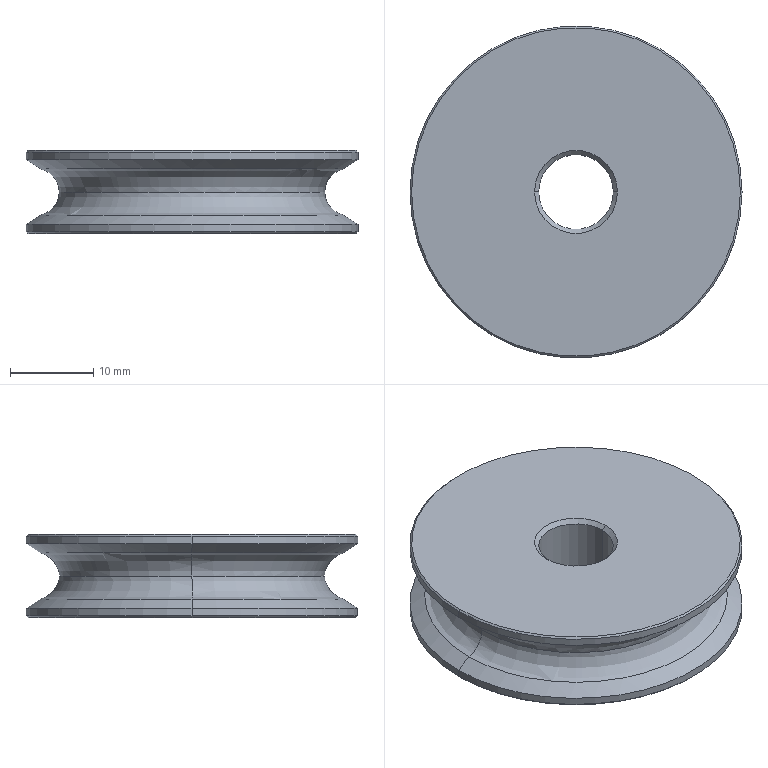Part | STEP file | 10000020591swp000-1 | 1 solid | 24 faces | box 40 x 40 x 10 mm | volume 9487 mm3 | cone 12 | cylinder 6 | torus 4 | plane 2 | commonest cylinder face diameters 40 x4 9 x2
STEP:
#1=CARTESIAN_POINT('',(-4.5,0.,4.5));
#2=VERTEX_POINT('',#1);
#3=CARTESIAN_POINT('',(4.5,0.,4.5));
#4=VERTEX_POINT('',#3);
#5=CARTESIAN_POINT('',(0.,0.,4.5));
#6=DIRECTION('',(0.,0.,1.));
#7=DIRECTION('',(1.,0.,0.));
#8=AXIS2_PLACEMENT_3D('',#5,#6,#7);
#9=CIRCLE('',#8,4.5);
#10=EDGE_CURVE('',#2,#4,#9,.T.);
#11=ORIENTED_EDGE('',*,*,#10,.F.);
#12=CARTESIAN_POINT('',(-5.,0.,5.));
#13=VERTEX_POINT('',#12);
#14=CARTESIAN_POINT('',(-4.5,0.,4.5));
#15=DIRECTION('',(-0.7071,0.,0.7071));
#16=VECTOR('',#15,1000.);
#17=LINE('',#14,#16);
#18=EDGE_CURVE('',#2,#13,#17,.T.);
#19=ORIENTED_EDGE('',*,*,#18,.T.);
#20=CARTESIAN_POINT('',(5.,0.,5.));
#21=VERTEX_POINT('',#20);
#22=CARTESIAN_POINT('',(0.,0.,5.));
#23=DIRECTION('',(0.,0.,-1.));
#24=DIRECTION('',(1.,0.,0.));
#25=AXIS2_PLACEMENT_3D('',#22,#23,#24);
#26=CIRCLE('',#25,5.);
#27=EDGE_CURVE('',#21,#13,#26,.T.);
#28=ORIENTED_EDGE('',*,*,#27,.F.);
#29=CARTESIAN_POINT('',(4.5,0.,4.5));
#30=DIRECTION('',(0.7071,0.,0.7071));
#31=VECTOR('',#30,1000.);
#32=LINE('',#29,#31);
#33=EDGE_CURVE('',#4,#21,#32,.T.);
#34=ORIENTED_EDGE('',*,*,#33,.F.);
#35=EDGE_LOOP('',(#11,#19,#28,#34));
#36=FACE_OUTER_BOUND('',#35,.T.);
#37=CARTESIAN_POINT('',(0.,0.,4.5));
#38=DIRECTION('',(0.,0.,1.));
#39=DIRECTION('',(1.,0.,0.));
#40=AXIS2_PLACEMENT_3D('',#37,#38,#39);
#41=CONICAL_SURFACE('',#40,4.5,0.7854);
#42=ADVANCED_FACE('',(#36),#41,.F.);
#43=CARTESIAN_POINT('',(4.5,0.,-4.5));
#44=VERTEX_POINT('',#43);
#45=CARTESIAN_POINT('',(-4.5,0.,-4.5));
#46=VERTEX_POINT('',#45);
#47=CARTESIAN_POINT('',(0.,0.,-4.5));
#48=DIRECTION('',(0.,0.,-1.));
#49=DIRECTION('',(1.,0.,0.));
#50=AXIS2_PLACEMENT_3D('',#47,#48,#49);
#51=CIRCLE('',#50,4.5);
#52=EDGE_CURVE('',#44,#46,#51,.T.);
#53=ORIENTED_EDGE('',*,*,#52,.F.);
#54=CARTESIAN_POINT('',(5.,0.,-5.));
#55=VERTEX_POINT('',#54);
#56=CARTESIAN_POINT('',(5.,0.,-5.));
#57=DIRECTION('',(0.7071,0.,-0.7071));
#58=VECTOR('',#57,1000.);
#59=LINE('',#56,#58);
#60=EDGE_CURVE('',#44,#55,#59,.T.);
#61=ORIENTED_EDGE('',*,*,#60,.T.);
#62=CARTESIAN_POINT('',(-5.,0.,-5.));
#63=VERTEX_POINT('',#62);
#64=CARTESIAN_POINT('',(0.,0.,-5.));
#65=DIRECTION('',(0.,0.,1.));
#66=DIRECTION('',(1.,0.,0.));
#67=AXIS2_PLACEMENT_3D('',#64,#65,#66);
#68=CIRCLE('',#67,5.);
#69=EDGE_CURVE('',#63,#55,#68,.T.);
#70=ORIENTED_EDGE('',*,*,#69,.F.);
#71=CARTESIAN_POINT('',(-5.,0.,-5.));
#72=DIRECTION('',(-0.7071,0.,-0.7071));
#73=VECTOR('',#72,1000.);
#74=LINE('',#71,#73);
#75=EDGE_CURVE('',#46,#63,#74,.T.);
#76=ORIENTED_EDGE('',*,*,#75,.F.);
#77=EDGE_LOOP('',(#53,#61,#70,#76));
#78=FACE_OUTER_BOUND('',#77,.T.);
#79=CARTESIAN_POINT('',(0.,0.,-5.));
#80=DIRECTION('',(0.,0.,-1.));
#81=DIRECTION('',(-1.,0.,0.));
#82=AXIS2_PLACEMENT_3D('',#79,#80,#81);
#83=CONICAL_SURFACE('',#82,5.,0.7854);
#84=ADVANCED_FACE('',(#78),#83,.F.);
#85=CARTESIAN_POINT('',(-19.8,0.,-5.));
#86=VERTEX_POINT('',#85);
#87=CARTESIAN_POINT('',(19.8,0.,-5.));
#88=VERTEX_POINT('',#87);
#89=CARTESIAN_POINT('',(0.,0.,-5.));
#90=DIRECTION('',(0.,0.,-1.));
#91=DIRECTION('',(1.,0.,0.));
#92=AXIS2_PLACEMENT_3D('',#89,#90,#91);
#93=CIRCLE('',#92,19.8);
#94=EDGE_CURVE('',#86,#88,#93,.T.);
#95=ORIENTED_EDGE('',*,*,#94,.F.);
#96=CARTESIAN_POINT('',(-20.,0.,-4.8));
#97=VERTEX_POINT('',#96);
#98=CARTESIAN_POINT('',(-20.,0.,-4.8));
#99=DIRECTION('',(-0.7071,0.,0.7071));
#100=VECTOR('',#99,1000.);
#101=LINE('',#98,#100);
#102=EDGE_CURVE('',#86,#97,#101,.T.);
#103=ORIENTED_EDGE('',*,*,#102,.T.);
#104=CARTESIAN_POINT('',(20.,0.,-4.8));
#105=VERTEX_POINT('',#104);
#106=CARTESIAN_POINT('',(0.,0.,-4.8));
#107=DIRECTION('',(0.,0.,1.));
#108=DIRECTION('',(1.,0.,0.));
#109=AXIS2_PLACEMENT_3D('',#106,#107,#108);
#110=CIRCLE('',#109,20.);
#111=EDGE_CURVE('',#105,#97,#110,.T.);
#112=ORIENTED_EDGE('',*,*,#111,.F.);
#113=CARTESIAN_POINT('',(20.,0.,-4.8));
#114=DIRECTION('',(0.7071,0.,0.7071));
#115=VECTOR('',#114,1000.);
#116=LINE('',#113,#115);
#117=EDGE_CURVE('',#88,#105,#116,.T.);
#118=ORIENTED_EDGE('',*,*,#117,.F.);
#119=EDGE_LOOP('',(#95,#103,#112,#118));
#120=FACE_OUTER_BOUND('',#119,.T.);
#121=CARTESIAN_POINT('',(0.,0.,-4.8));
#122=DIRECTION('',(0.,0.,1.));
#123=DIRECTION('',(1.,0.,0.));
#124=AXIS2_PLACEMENT_3D('',#121,#122,#123);
#125=CONICAL_SURFACE('',#124,20.,0.7854);
#126=ADVANCED_FACE('',(#120),#125,.T.);
#127=CARTESIAN_POINT('',(19.8,0.,5.));
#128=VERTEX_POINT('',#127);
#129=CARTESIAN_POINT('',(-19.8,0.,5.));
#130=VERTEX_POINT('',#129);
#131=CARTESIAN_POINT('',(0.,0.,5.));
#132=DIRECTION('',(0.,0.,1.));
#133=DIRECTION('',(1.,0.,0.));
#134=AXIS2_PLACEMENT_3D('',#131,#132,#133);
#135=CIRCLE('',#134,19.8);
#136=EDGE_CURVE('',#128,#130,#135,.T.);
#137=ORIENTED_EDGE('',*,*,#136,.F.);
#138=CARTESIAN_POINT('',(20.,0.,4.8));
#139=VERTEX_POINT('',#138);
#140=CARTESIAN_POINT('',(19.8,0.,5.));
#141=DIRECTION('',(0.7071,0.,-0.7071));
#142=VECTOR('',#141,1000.);
#143=LINE('',#140,#142);
#144=EDGE_CURVE('',#128,#139,#143,.T.);
#145=ORIENTED_EDGE('',*,*,#144,.T.);
#146=CARTESIAN_POINT('',(-20.,0.,4.8));
#147=VERTEX_POINT('',#146);
#148=CARTESIAN_POINT('',(0.,0.,4.8));
#149=DIRECTION('',(0.,0.,-1.));
#150=DIRECTION('',(1.,0.,0.));
#151=AXIS2_PLACEMENT_3D('',#148,#149,#150);
#152=CIRCLE('',#151,20.);
#153=EDGE_CURVE('',#147,#139,#152,.T.);
#154=ORIENTED_EDGE('',*,*,#153,.F.);
#155=CARTESIAN_POINT('',(-19.8,0.,5.));
#156=DIRECTION('',(-0.7071,0.,-0.7071));
#157=VECTOR('',#156,1000.);
#158=LINE('',#155,#157);
#159=EDGE_CURVE('',#130,#147,#158,.T.);
#160=ORIENTED_EDGE('',*,*,#159,.F.);
#161=EDGE_LOOP('',(#137,#145,#154,#160));
#162=FACE_OUTER_BOUND('',#161,.T.);
#163=CARTESIAN_POINT('',(0.,0.,5.));
#164=DIRECTION('',(0.,0.,-1.));
#165=DIRECTION('',(-1.,0.,0.));
#166=AXIS2_PLACEMENT_3D('',#163,#164,#165);
#167=CONICAL_SURFACE('',#166,19.8,0.7854);
#168=ADVANCED_FACE('',(#162),#167,.T.);
#169=CARTESIAN_POINT('',(-18.244,0.,2.785));
#170=VERTEX_POINT('',#169);
#171=CARTESIAN_POINT('',(18.244,0.,2.785));
#172=VERTEX_POINT('',#171);
#173=CARTESIAN_POINT('',(0.,0.,2.785));
#174=DIRECTION('',(0.,0.,-1.));
#175=DIRECTION('',(-1.,0.,0.));
#176=AXIS2_PLACEMENT_3D('',#173,#174,#175);
#177=CIRCLE('',#176,18.244);
#178=EDGE_CURVE('',#170,#172,#177,.T.);
#179=ORIENTED_EDGE('',*,*,#178,.F.);
#180=CARTESIAN_POINT('',(-20.,0.,3.909));
#181=VERTEX_POINT('',#180);
#182=CARTESIAN_POINT('',(-20.,0.,3.909));
#183=DIRECTION('',(-0.8422,0.,0.5391));
#184=VECTOR('',#183,1000.);
#185=LINE('',#182,#184);
#186=EDGE_CURVE('',#170,#181,#185,.T.);
#187=ORIENTED_EDGE('',*,*,#186,.T.);
#188=CARTESIAN_POINT('',(20.,0.,3.909));
#189=VERTEX_POINT('',#188);
#190=CARTESIAN_POINT('',(0.,0.,3.909));
#191=DIRECTION('',(0.,0.,1.));
#192=DIRECTION('',(1.,0.,0.));
#193=AXIS2_PLACEMENT_3D('',#190,#191,#192);
#194=CIRCLE('',#193,20.);
#195=EDGE_CURVE('',#189,#181,#194,.T.);
#196=ORIENTED_EDGE('',*,*,#195,.F.);
#197=CARTESIAN_POINT('',(20.,0.,3.909));
#198=DIRECTION('',(0.8422,0.,0.5391));
#199=VECTOR('',#198,1000.);
#200=LINE('',#197,#199);
#201=EDGE_CURVE('',#172,#189,#200,.T.);
#202=ORIENTED_EDGE('',*,*,#201,.F.);
#203=EDGE_LOOP('',(#179,#187,#196,#202));
#204=FACE_OUTER_BOUND('',#203,.T.);
#205=CARTESIAN_POINT('',(0.,0.,3.909));
#206=DIRECTION('',(0.,0.,1.));
#207=DIRECTION('',(1.,0.,0.));
#208=AXIS2_PLACEMENT_3D('',#205,#206,#207);
#209=CONICAL_SURFACE('',#208,20.,1.001);
#210=ADVANCED_FACE('',(#204),#209,.T.);
#211=CARTESIAN_POINT('',(18.244,0.,-2.785));
#212=VERTEX_POINT('',#211);
#213=CARTESIAN_POINT('',(-18.244,0.,-2.785));
#214=VERTEX_POINT('',#213);
#215=CARTESIAN_POINT('',(0.,0.,-2.785));
#216=DIRECTION('',(0.,0.,1.));
#217=DIRECTION('',(1.,0.,0.));
#218=AXIS2_PLACEMENT_3D('',#215,#216,#217);
#219=CIRCLE('',#218,18.244);
#220=EDGE_CURVE('',#212,#214,#219,.T.);
#221=ORIENTED_EDGE('',*,*,#220,.F.);
#222=CARTESIAN_POINT('',(20.,0.,-3.909));
#223=VERTEX_POINT('',#222);
#224=CARTESIAN_POINT('',(18.244,0.,-2.785));
#225=DIRECTION('',(0.8422,0.,-0.5391));
#226=VECTOR('',#225,1000.);
#227=LINE('',#224,#226);
#228=EDGE_CURVE('',#212,#223,#227,.T.);
#229=ORIENTED_EDGE('',*,*,#228,.T.);
#230=CARTESIAN_POINT('',(-20.,0.,-3.909));
#231=VERTEX_POINT('',#230);
#232=CARTESIAN_POINT('',(0.,0.,-3.909));
#233=DIRECTION('',(0.,0.,-1.));
#234=DIRECTION('',(-1.,0.,0.));
#235=AXIS2_PLACEMENT_3D('',#232,#233,#234);
#236=CIRCLE('',#235,20.);
#237=EDGE_CURVE('',#231,#223,#236,.T.);
#238=ORIENTED_EDGE('',*,*,#237,.F.);
#239=CARTESIAN_POINT('',(-18.244,0.,-2.785));
#240=DIRECTION('',(-0.8422,0.,-0.5391));
#241=VECTOR('',#240,1000.);
#242=LINE('',#239,#241);
#243=EDGE_CURVE('',#214,#231,#242,.T.);
#244=ORIENTED_EDGE('',*,*,#243,.F.);
#245=EDGE_LOOP('',(#221,#229,#238,#244));
#246=FACE_OUTER_BOUND('',#245,.T.);
#247=CARTESIAN_POINT('',(0.,0.,-2.785));
#248=DIRECTION('',(0.,0.,-1.));
#249=DIRECTION('',(-1.,0.,0.));
#250=AXIS2_PLACEMENT_3D('',#247,#248,#249);
#251=CONICAL_SURFACE('',#250,18.244,1.001);
#252=ADVANCED_FACE('',(#246),#251,.T.);
#253=CARTESIAN_POINT('',(0.,0.,-2.785));
#254=DIRECTION('',(0.,0.,1.));
#255=DIRECTION('',(1.,0.,0.));
#256=AXIS2_PLACEMENT_3D('',#253,#254,#255);
#257=CIRCLE('',#256,18.244);
#258=EDGE_CURVE('',#214,#212,#257,.T.);
#259=ORIENTED_EDGE('',*,*,#258,.T.);
#260=CARTESIAN_POINT('',(16.,0.,0.));
#261=VERTEX_POINT('',#260);
#262=CARTESIAN_POINT('',(18.85,0.,0.));
#263=DIRECTION('',(0.,1.,0.));
#264=DIRECTION('',(-1.,0.,0.));
#265=AXIS2_PLACEMENT_3D('',#262,#263,#264);
#266=CIRCLE('',#265,2.85);
#267=EDGE_CURVE('',#212,#261,#266,.T.);
#268=ORIENTED_EDGE('',*,*,#267,.T.);
#269=CARTESIAN_POINT('',(-16.,0.,0.));
#270=VERTEX_POINT('',#269);
#271=CARTESIAN_POINT('',(0.,0.,0.));
#272=DIRECTION('',(0.,0.,-1.));
#273=DIRECTION('',(1.,0.,0.));
#274=AXIS2_PLACEMENT_3D('',#271,#272,#273);
#275=CIRCLE('',#274,16.);
#276=EDGE_CURVE('',#261,#270,#275,.T.);
#277=ORIENTED_EDGE('',*,*,#276,.T.);
#278=CARTESIAN_POINT('',(-18.85,0.,0.));
#279=DIRECTION('',(0.,-1.,0.));
#280=DIRECTION('',(0.,0.,-1.));
#281=AXIS2_PLACEMENT_3D('',#278,#279,#280);
#282=CIRCLE('',#281,2.85);
#283=EDGE_CURVE('',#214,#270,#282,.T.);
#284=ORIENTED_EDGE('',*,*,#283,.F.);
#285=EDGE_LOOP('',(#259,#268,#277,#284));
#286=FACE_OUTER_BOUND('',#285,.T.);
#287=CARTESIAN_POINT('',(0.,0.,0.));
#288=DIRECTION('',(0.,0.,-1.));
#289=DIRECTION('',(-1.,0.,0.));
#290=AXIS2_PLACEMENT_3D('',#287,#288,#289);
#291=TOROIDAL_SURFACE('',#290,18.85,2.85);
#292=ADVANCED_FACE('',(#286),#291,.F.);
#293=CARTESIAN_POINT('',(0.,0.,2.785));
#294=DIRECTION('',(0.,0.,-1.));
#295=DIRECTION('',(-1.,0.,0.));
#296=AXIS2_PLACEMENT_3D('',#293,#294,#295);
#297=CIRCLE('',#296,18.244);
#298=EDGE_CURVE('',#172,#170,#297,.T.);
#299=ORIENTED_EDGE('',*,*,#298,.T.);
#300=CARTESIAN_POINT('',(-18.85,0.,0.));
#301=DIRECTION('',(0.,1.,0.));
#302=DIRECTION('',(-1.,0.,0.));
#303=AXIS2_PLACEMENT_3D('',#300,#301,#302);
#304=CIRCLE('',#303,2.85);
#305=EDGE_CURVE('',#170,#270,#304,.T.);
#306=ORIENTED_EDGE('',*,*,#305,.T.);
#307=ORIENTED_EDGE('',*,*,#276,.F.);
#308=CARTESIAN_POINT('',(18.85,0.,0.));
#309=DIRECTION('',(0.,-1.,0.));
#310=DIRECTION('',(0.,0.,-1.));
#311=AXIS2_PLACEMENT_3D('',#308,#309,#310);
#312=CIRCLE('',#311,2.85);
#313=EDGE_CURVE('',#172,#261,#312,.T.);
#314=ORIENTED_EDGE('',*,*,#313,.F.);
#315=EDGE_LOOP('',(#299,#306,#307,#314));
#316=FACE_OUTER_BOUND('',#315,.T.);
#317=CARTESIAN_POINT('',(0.,0.,0.));
#318=DIRECTION('',(0.,0.,1.));
#319=DIRECTION('',(1.,0.,0.));
#320=AXIS2_PLACEMENT_3D('',#317,#318,#319);
#321=TOROIDAL_SURFACE('',#320,18.85,2.85);
#322=ADVANCED_FACE('',(#316),#321,.F.);
#323=ORIENTED_EDGE('',*,*,#52,.T.);
#324=CARTESIAN_POINT('',(-4.5,0.,5.));
#325=DIRECTION('',(0.,0.,1.));
#326=VECTOR('',#325,1000.);
#327=LINE('',#324,#326);
#328=EDGE_CURVE('',#46,#2,#327,.T.);
#329=ORIENTED_EDGE('',*,*,#328,.T.);
#330=ORIENTED_EDGE('',*,*,#10,.T.);
#331=CARTESIAN_POINT('',(4.5,0.,5.));
#332=DIRECTION('',(0.,0.,1.));
#333=VECTOR('',#332,1000.);
#334=LINE('',#331,#333);
#335=EDGE_CURVE('',#44,#4,#334,.T.);
#336=ORIENTED_EDGE('',*,*,#335,.F.);
#337=EDGE_LOOP('',(#323,#329,#330,#336));
#338=FACE_OUTER_BOUND('',#337,.T.);
#339=CARTESIAN_POINT('',(0.,0.,5.));
#340=DIRECTION('',(0.,0.,1.));
#341=DIRECTION('',(1.,0.,0.));
#342=AXIS2_PLACEMENT_3D('',#339,#340,#341);
#343=CYLINDRICAL_SURFACE('',#342,4.5);
#344=ADVANCED_FACE('',(#338),#343,.F.);
#345=ORIENTED_EDGE('',*,*,#237,.T.);
#346=CARTESIAN_POINT('',(20.,0.,5.));
#347=DIRECTION('',(0.,0.,-1.));
#348=VECTOR('',#347,1000.);
#349=LINE('',#346,#348);
#350=EDGE_CURVE('',#223,#105,#349,.T.);
#351=ORIENTED_EDGE('',*,*,#350,.T.);
#352=ORIENTED_EDGE('',*,*,#111,.T.);
#353=CARTESIAN_POINT('',(-20.,0.,5.));
#354=DIRECTION('',(0.,0.,-1.));
#355=VECTOR('',#354,1000.);
#356=LINE('',#353,#355);
#357=EDGE_CURVE('',#231,#97,#356,.T.);
#358=ORIENTED_EDGE('',*,*,#357,.F.);
#359=EDGE_LOOP('',(#345,#351,#352,#358));
#360=FACE_OUTER_BOUND('',#359,.T.);
#361=CARTESIAN_POINT('',(0.,0.,5.));
#362=DIRECTION('',(0.,0.,-1.));
#363=DIRECTION('',(-1.,0.,0.));
#364=AXIS2_PLACEMENT_3D('',#361,#362,#363);
#365=CYLINDRICAL_SURFACE('',#364,20.);
#366=ADVANCED_FACE('',(#360),#365,.T.);
#367=ORIENTED_EDGE('',*,*,#153,.T.);
#368=CARTESIAN_POINT('',(20.,0.,5.));
#369=DIRECTION('',(0.,0.,-1.));
#370=VECTOR('',#369,1000.);
#371=LINE('',#368,#370);
#372=EDGE_CURVE('',#139,#189,#371,.T.);
#373=ORIENTED_EDGE('',*,*,#372,.T.);
#374=ORIENTED_EDGE('',*,*,#195,.T.);
#375=CARTESIAN_POINT('',(-20.,0.,5.));
#376=DIRECTION('',(0.,0.,-1.));
#377=VECTOR('',#376,1000.);
#378=LINE('',#375,#377);
#379=EDGE_CURVE('',#147,#181,#378,.T.);
#380=ORIENTED_EDGE('',*,*,#379,.F.);
#381=EDGE_LOOP('',(#367,#373,#374,#380));
#382=FACE_OUTER_BOUND('',#381,.T.);
#383=CARTESIAN_POINT('',(0.,0.,5.));
#384=DIRECTION('',(0.,0.,-1.));
#385=DIRECTION('',(-1.,0.,0.));
#386=AXIS2_PLACEMENT_3D('',#383,#384,#385);
#387=CYLINDRICAL_SURFACE('',#386,20.);
#388=ADVANCED_FACE('',(#382),#387,.T.);
#389=ORIENTED_EDGE('',*,*,#372,.F.);
#390=CARTESIAN_POINT('',(0.,0.,4.8));
#391=DIRECTION('',(0.,0.,-1.));
#392=DIRECTION('',(1.,0.,0.));
#393=AXIS2_PLACEMENT_3D('',#390,#391,#392);
#394=CIRCLE('',#393,20.);
#395=EDGE_CURVE('',#139,#147,#394,.T.);
#396=ORIENTED_EDGE('',*,*,#395,.T.);
#397=ORIENTED_EDGE('',*,*,#379,.T.);
#398=CARTESIAN_POINT('',(0.,0.,3.909));
#399=DIRECTION('',(0.,0.,1.));
#400=DIRECTION('',(1.,0.,0.));
#401=AXIS2_PLACEMENT_3D('',#398,#399,#400);
#402=CIRCLE('',#401,20.);
#403=EDGE_CURVE('',#181,#189,#402,.T.);
#404=ORIENTED_EDGE('',*,*,#403,.T.);
#405=EDGE_LOOP('',(#389,#396,#397,#404));
#406=FACE_OUTER_BOUND('',#405,.T.);
#407=CARTESIAN_POINT('',(0.,0.,5.));
#408=DIRECTION('',(0.,0.,-1.));
#409=DIRECTION('',(-1.,0.,0.));
#410=AXIS2_PLACEMENT_3D('',#407,#408,#409);
#411=CYLINDRICAL_SURFACE('',#410,20.);
#412=ADVANCED_FACE('',(#406),#411,.T.);
#413=ORIENTED_EDGE('',*,*,#350,.F.);
#414=CARTESIAN_POINT('',(0.,0.,-3.909));
#415=DIRECTION('',(0.,0.,-1.));
#416=DIRECTION('',(-1.,0.,0.));
#417=AXIS2_PLACEMENT_3D('',#414,#415,#416);
#418=CIRCLE('',#417,20.);
#419=EDGE_CURVE('',#223,#231,#418,.T.);
#420=ORIENTED_EDGE('',*,*,#419,.T.);
#421=ORIENTED_EDGE('',*,*,#357,.T.);
#422=CARTESIAN_POINT('',(0.,0.,-4.8));
#423=DIRECTION('',(0.,0.,1.));
#424=DIRECTION('',(1.,0.,0.));
#425=AXIS2_PLACEMENT_3D('',#422,#423,#424);
#426=CIRCLE('',#425,20.);
#427=EDGE_CURVE('',#97,#105,#426,.T.);
#428=ORIENTED_EDGE('',*,*,#427,.T.);
#429=EDGE_LOOP('',(#413,#420,#421,#428));
#430=FACE_OUTER_BOUND('',#429,.T.);
#431=CARTESIAN_POINT('',(0.,0.,5.));
#432=DIRECTION('',(0.,0.,-1.));
#433=DIRECTION('',(-1.,0.,0.));
#434=AXIS2_PLACEMENT_3D('',#431,#432,#433);
#435=CYLINDRICAL_SURFACE('',#434,20.);
#436=ADVANCED_FACE('',(#430),#435,.T.);
#437=ORIENTED_EDGE('',*,*,#27,.T.);
#438=CARTESIAN_POINT('',(0.,0.,5.));
#439=DIRECTION('',(0.,0.,-1.));
#440=DIRECTION('',(1.,0.,0.));
#441=AXIS2_PLACEMENT_3D('',#438,#439,#440);
#442=CIRCLE('',#441,5.);
#443=EDGE_CURVE('',#13,#21,#442,.T.);
#444=ORIENTED_EDGE('',*,*,#443,.T.);
#445=EDGE_LOOP('',(#437,#444));
#446=FACE_BOUND('',#445,.T.);
#447=CARTESIAN_POINT('',(0.,0.,5.));
#448=DIRECTION('',(0.,0.,1.));
#449=DIRECTION('',(1.,0.,0.));
#450=AXIS2_PLACEMENT_3D('',#447,#448,#449);
#451=CIRCLE('',#450,19.8);
#452=EDGE_CURVE('',#130,#128,#451,.T.);
#453=ORIENTED_EDGE('',*,*,#452,.T.);
#454=ORIENTED_EDGE('',*,*,#136,.T.);
#455=EDGE_LOOP('',(#453,#454));
#456=FACE_OUTER_BOUND('',#455,.T.);
#457=CARTESIAN_POINT('',(0.,0.,5.));
#458=DIRECTION('',(0.,0.,1.));
#459=DIRECTION('',(1.,0.,0.));
#460=AXIS2_PLACEMENT_3D('',#457,#458,#459);
#461=PLANE('',#460);
#462=ADVANCED_FACE('',(#446,#456),#461,.T.);
#463=ORIENTED_EDGE('',*,*,#69,.T.);
#464=CARTESIAN_POINT('',(0.,0.,-5.));
#465=DIRECTION('',(0.,0.,1.));
#466=DIRECTION('',(1.,0.,0.));
#467=AXIS2_PLACEMENT_3D('',#464,#465,#466);
#468=CIRCLE('',#467,5.);
#469=EDGE_CURVE('',#55,#63,#468,.T.);
#470=ORIENTED_EDGE('',*,*,#469,.T.);
#471=EDGE_LOOP('',(#463,#470));
#472=FACE_BOUND('',#471,.T.);
#473=CARTESIAN_POINT('',(0.,0.,-5.));
#474=DIRECTION('',(0.,0.,-1.));
#475=DIRECTION('',(1.,0.,0.));
#476=AXIS2_PLACEMENT_3D('',#473,#474,#475);
#477=CIRCLE('',#476,19.8);
#478=EDGE_CURVE('',#88,#86,#477,.T.);
#479=ORIENTED_EDGE('',*,*,#478,.T.);
#480=ORIENTED_EDGE('',*,*,#94,.T.);
#481=EDGE_LOOP('',(#479,#480));
#482=FACE_OUTER_BOUND('',#481,.T.);
#483=CARTESIAN_POINT('',(0.,0.,-5.));
#484=DIRECTION('',(0.,0.,1.));
#485=DIRECTION('',(1.,0.,0.));
#486=AXIS2_PLACEMENT_3D('',#483,#484,#485);
#487=PLANE('',#486);
#488=ADVANCED_FACE('',(#472,#482),#487,.F.);
#489=ORIENTED_EDGE('',*,*,#328,.F.);
#490=CARTESIAN_POINT('',(0.,0.,-4.5));
#491=DIRECTION('',(0.,0.,-1.));
#492=DIRECTION('',(1.,0.,0.));
#493=AXIS2_PLACEMENT_3D('',#490,#491,#492);
#494=CIRCLE('',#493,4.5);
#495=EDGE_CURVE('',#46,#44,#494,.T.);
#496=ORIENTED_EDGE('',*,*,#495,.T.);
#497=ORIENTED_EDGE('',*,*,#335,.T.);
#498=CARTESIAN_POINT('',(0.,0.,4.5));
#499=DIRECTION('',(0.,0.,1.));
#500=DIRECTION('',(1.,0.,0.));
#501=AXIS2_PLACEMENT_3D('',#498,#499,#500);
#502=CIRCLE('',#501,4.5);
#503=EDGE_CURVE('',#4,#2,#502,.T.);
#504=ORIENTED_EDGE('',*,*,#503,.T.);
#505=EDGE_LOOP('',(#489,#496,#497,#504));
#506=FACE_OUTER_BOUND('',#505,.T.);
#507=CARTESIAN_POINT('',(0.,0.,5.));
#508=DIRECTION('',(0.,0.,1.));
#509=DIRECTION('',(1.,0.,0.));
#510=AXIS2_PLACEMENT_3D('',#507,#508,#509);
#511=CYLINDRICAL_SURFACE('',#510,4.5);
#512=ADVANCED_FACE('',(#506),#511,.F.);
#513=ORIENTED_EDGE('',*,*,#305,.F.);
#514=ORIENTED_EDGE('',*,*,#178,.T.);
#515=ORIENTED_EDGE('',*,*,#313,.T.);
#516=CARTESIAN_POINT('',(0.,0.,0.));
#517=DIRECTION('',(0.,0.,-1.));
#518=DIRECTION('',(1.,0.,0.));
#519=AXIS2_PLACEMENT_3D('',#516,#517,#518);
#520=CIRCLE('',#519,16.);
#521=EDGE_CURVE('',#270,#261,#520,.T.);
#522=ORIENTED_EDGE('',*,*,#521,.F.);
#523=EDGE_LOOP('',(#513,#514,#515,#522));
#524=FACE_OUTER_BOUND('',#523,.T.);
#525=CARTESIAN_POINT('',(0.,0.,0.));
#526=DIRECTION('',(0.,0.,1.));
#527=DIRECTION('',(1.,0.,0.));
#528=AXIS2_PLACEMENT_3D('',#525,#526,#527);
#529=TOROIDAL_SURFACE('',#528,18.85,2.85);
#530=ADVANCED_FACE('',(#524),#529,.F.);
#531=ORIENTED_EDGE('',*,*,#267,.F.);
#532=ORIENTED_EDGE('',*,*,#220,.T.);
#533=ORIENTED_EDGE('',*,*,#283,.T.);
#534=ORIENTED_EDGE('',*,*,#521,.T.);
#535=EDGE_LOOP('',(#531,#532,#533,#534));
#536=FACE_OUTER_BOUND('',#535,.T.);
#537=CARTESIAN_POINT('',(0.,0.,0.));
#538=DIRECTION('',(0.,0.,-1.));
#539=DIRECTION('',(-1.,0.,0.));
#540=AXIS2_PLACEMENT_3D('',#537,#538,#539);
#541=TOROIDAL_SURFACE('',#540,18.85,2.85);
#542=ADVANCED_FACE('',(#536),#541,.F.);
#543=ORIENTED_EDGE('',*,*,#228,.F.);
#544=ORIENTED_EDGE('',*,*,#258,.F.);
#545=ORIENTED_EDGE('',*,*,#243,.T.);
#546=ORIENTED_EDGE('',*,*,#419,.F.);
#547=EDGE_LOOP('',(#543,#544,#545,#546));
#548=FACE_OUTER_BOUND('',#547,.T.);
#549=CARTESIAN_POINT('',(0.,0.,-2.785));
#550=DIRECTION('',(0.,0.,-1.));
#551=DIRECTION('',(-1.,0.,0.));
#552=AXIS2_PLACEMENT_3D('',#549,#550,#551);
#553=CONICAL_SURFACE('',#552,18.244,1.001);
#554=ADVANCED_FACE('',(#548),#553,.T.);
#555=ORIENTED_EDGE('',*,*,#186,.F.);
#556=ORIENTED_EDGE('',*,*,#298,.F.);
#557=ORIENTED_EDGE('',*,*,#201,.T.);
#558=ORIENTED_EDGE('',*,*,#403,.F.);
#559=EDGE_LOOP('',(#555,#556,#557,#558));
#560=FACE_OUTER_BOUND('',#559,.T.);
#561=CARTESIAN_POINT('',(0.,0.,3.909));
#562=DIRECTION('',(0.,0.,1.));
#563=DIRECTION('',(1.,0.,0.));
#564=AXIS2_PLACEMENT_3D('',#561,#562,#563);
#565=CONICAL_SURFACE('',#564,20.,1.001);
#566=ADVANCED_FACE('',(#560),#565,.T.);
#567=ORIENTED_EDGE('',*,*,#144,.F.);
#568=ORIENTED_EDGE('',*,*,#452,.F.);
#569=ORIENTED_EDGE('',*,*,#159,.T.);
#570=ORIENTED_EDGE('',*,*,#395,.F.);
#571=EDGE_LOOP('',(#567,#568,#569,#570));
#572=FACE_OUTER_BOUND('',#571,.T.);
#573=CARTESIAN_POINT('',(0.,0.,5.));
#574=DIRECTION('',(0.,0.,-1.));
#575=DIRECTION('',(-1.,0.,0.));
#576=AXIS2_PLACEMENT_3D('',#573,#574,#575);
#577=CONICAL_SURFACE('',#576,19.8,0.7854);
#578=ADVANCED_FACE('',(#572),#577,.T.);
#579=ORIENTED_EDGE('',*,*,#102,.F.);
#580=ORIENTED_EDGE('',*,*,#478,.F.);
#581=ORIENTED_EDGE('',*,*,#117,.T.);
#582=ORIENTED_EDGE('',*,*,#427,.F.);
#583=EDGE_LOOP('',(#579,#580,#581,#582));
#584=FACE_OUTER_BOUND('',#583,.T.);
#585=CARTESIAN_POINT('',(0.,0.,-4.8));
#586=DIRECTION('',(0.,0.,1.));
#587=DIRECTION('',(1.,0.,0.));
#588=AXIS2_PLACEMENT_3D('',#585,#586,#587);
#589=CONICAL_SURFACE('',#588,20.,0.7854);
#590=ADVANCED_FACE('',(#584),#589,.T.);
#591=ORIENTED_EDGE('',*,*,#60,.F.);
#592=ORIENTED_EDGE('',*,*,#495,.F.);
#593=ORIENTED_EDGE('',*,*,#75,.T.);
#594=ORIENTED_EDGE('',*,*,#469,.F.);
#595=EDGE_LOOP('',(#591,#592,#593,#594));
#596=FACE_OUTER_BOUND('',#595,.T.);
#597=CARTESIAN_POINT('',(0.,0.,-5.));
#598=DIRECTION('',(0.,0.,-1.));
#599=DIRECTION('',(-1.,0.,0.));
#600=AXIS2_PLACEMENT_3D('',#597,#598,#599);
#601=CONICAL_SURFACE('',#600,5.,0.7854);
#602=ADVANCED_FACE('',(#596),#601,.F.);
#603=ORIENTED_EDGE('',*,*,#18,.F.);
#604=ORIENTED_EDGE('',*,*,#503,.F.);
#605=ORIENTED_EDGE('',*,*,#33,.T.);
#606=ORIENTED_EDGE('',*,*,#443,.F.);
#607=EDGE_LOOP('',(#603,#604,#605,#606));
#608=FACE_OUTER_BOUND('',#607,.T.);
#609=CARTESIAN_POINT('',(0.,0.,4.5));
#610=DIRECTION('',(0.,0.,1.));
#611=DIRECTION('',(1.,0.,0.));
#612=AXIS2_PLACEMENT_3D('',#609,#610,#611);
#613=CONICAL_SURFACE('',#612,4.5,0.7854);
#614=ADVANCED_FACE('',(#608),#613,.F.);
#615=CLOSED_SHELL('',(#42,#84,#126,#168,#210,#252,#292,#322,#344,#366,#388,#412,#436,#462,#488,#512,#530,#542,#554,#566,#578,#590,#602,#614));
#616=MANIFOLD_SOLID_BREP('',#615);
#617=CARTESIAN_POINT('',(0.,0.,0.));
#618=DIRECTION('',(0.,0.,1.));
#619=DIRECTION('',(1.,0.,0.));
#620=AXIS2_PLACEMENT_3D('',#617,#618,#619);
#621=(LENGTH_UNIT()NAMED_UNIT(*)SI_UNIT(.MILLI.,.METRE.));
#622=UNCERTAINTY_MEASURE_WITH_UNIT(LENGTH_MEASURE(0.00001),#621,'','');
#623=(NAMED_UNIT(*)PLANE_ANGLE_UNIT()SI_UNIT($,.RADIAN.));
#624=(NAMED_UNIT(*)SI_UNIT($,.STERADIAN.)SOLID_ANGLE_UNIT());
#625=(GEOMETRIC_REPRESENTATION_CONTEXT(3)GLOBAL_UNCERTAINTY_ASSIGNED_CONTEXT((#622))GLOBAL_UNIT_ASSIGNED_CONTEXT((#621,#623,#624))REPRESENTATION_CONTEXT('',''));
#626=ADVANCED_BREP_SHAPE_REPRESENTATION('',(#616,#620),#625);